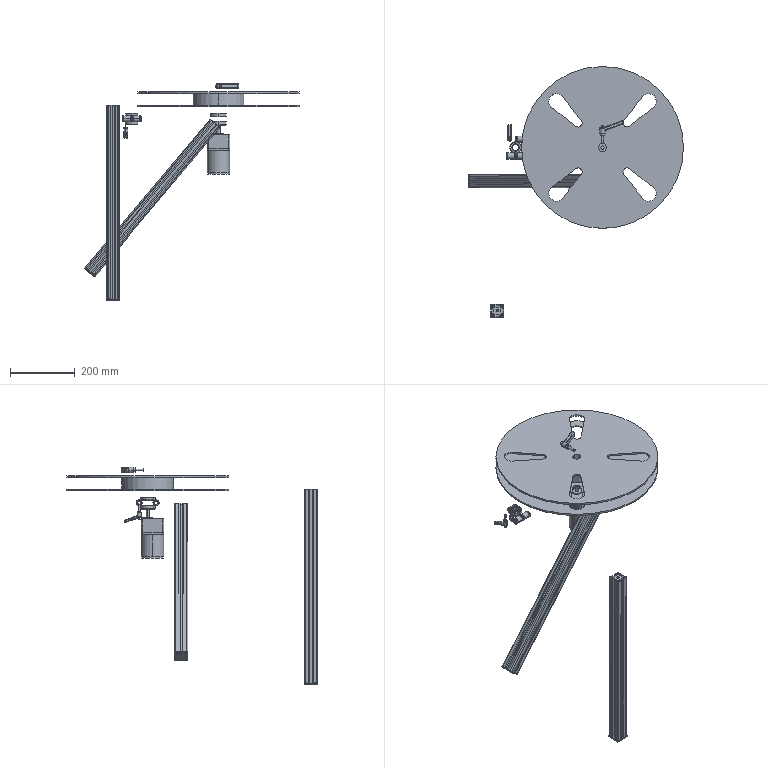Part | NX | 15 solids | 675 faces | box 663.862 x 774 x 671.72 mm | volume 4156417 mm3 | cylinder 260 | plane 258 | cone 68 | torus 57 | spline 22 | sphere 10 | commonest cylinder face diameters 8 x34 10 x18 19 x18 25 x18 1 x16 5.5 x16